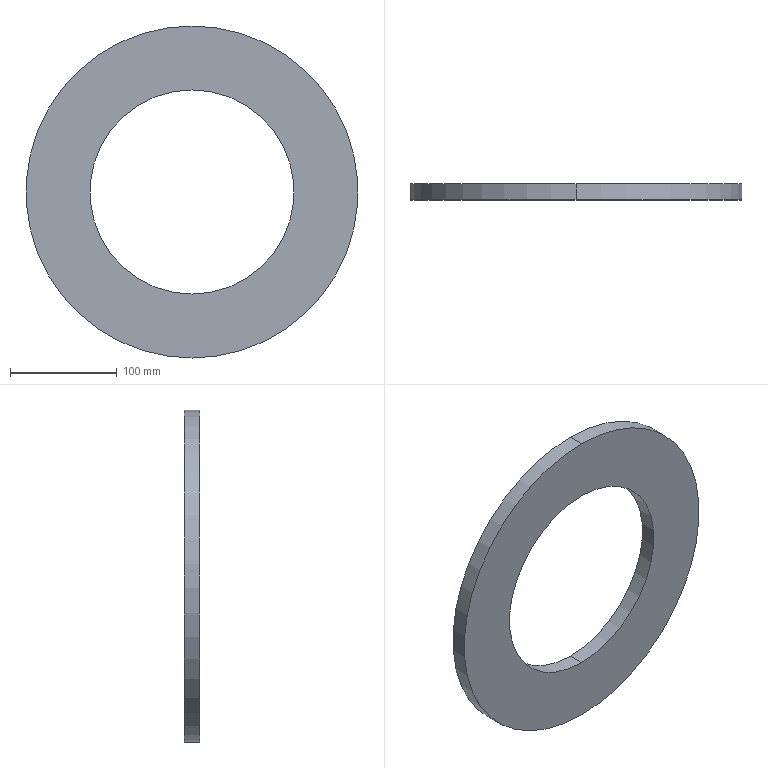Part | SolidWorks | features Extrusion 1 | 1 solid | 6 faces | box 311.64 x 15 x 311.64 mm | volume 711495 mm3 | cylinder 4 | plane 2 | commonest cylinder face diameters 191.64 x2 311.64 x2
STEP:
#1=CARTESIAN_POINT('',(0.,15.,-95.82));
#2=VERTEX_POINT('',#1);
#3=CARTESIAN_POINT('',(0.,15.,95.82));
#4=VERTEX_POINT('',#3);
#5=CARTESIAN_POINT('',(0.,15.,0.));
#6=DIRECTION('',(0.,1.,0.));
#7=DIRECTION('',(0.,0.,1.));
#8=AXIS2_PLACEMENT_3D('',#5,#6,#7);
#9=CIRCLE('',#8,95.82);
#10=EDGE_CURVE('',#2,#4,#9,.T.);
#11=ORIENTED_EDGE('',*,*,#10,.T.);
#12=CARTESIAN_POINT('',(0.,0.,95.82));
#13=VERTEX_POINT('',#12);
#14=CARTESIAN_POINT('',(0.,15.,95.82));
#15=DIRECTION('',(0.,-1.,0.));
#16=VECTOR('',#15,1000.);
#17=LINE('',#14,#16);
#18=EDGE_CURVE('',#4,#13,#17,.T.);
#19=ORIENTED_EDGE('',*,*,#18,.T.);
#20=CARTESIAN_POINT('',(0.,0.,-95.82));
#21=VERTEX_POINT('',#20);
#22=CARTESIAN_POINT('',(0.,0.,0.));
#23=DIRECTION('',(0.,1.,0.));
#24=DIRECTION('',(0.,0.,1.));
#25=AXIS2_PLACEMENT_3D('',#22,#23,#24);
#26=CIRCLE('',#25,95.82);
#27=EDGE_CURVE('',#21,#13,#26,.T.);
#28=ORIENTED_EDGE('',*,*,#27,.F.);
#29=CARTESIAN_POINT('',(0.,15.,-95.82));
#30=DIRECTION('',(0.,-1.,0.));
#31=VECTOR('',#30,1000.);
#32=LINE('',#29,#31);
#33=EDGE_CURVE('',#2,#21,#32,.T.);
#34=ORIENTED_EDGE('',*,*,#33,.F.);
#35=EDGE_LOOP('',(#11,#19,#28,#34));
#36=FACE_OUTER_BOUND('',#35,.T.);
#37=CARTESIAN_POINT('',(0.,15.,0.));
#38=DIRECTION('',(0.,-1.,0.));
#39=DIRECTION('',(0.,0.,-1.));
#40=AXIS2_PLACEMENT_3D('',#37,#38,#39);
#41=CYLINDRICAL_SURFACE('',#40,95.82);
#42=ADVANCED_FACE('',(#36),#41,.F.);
#43=CARTESIAN_POINT('',(0.,15.,155.82));
#44=VERTEX_POINT('',#43);
#45=CARTESIAN_POINT('',(0.,15.,-155.82));
#46=VERTEX_POINT('',#45);
#47=CARTESIAN_POINT('',(0.,15.,0.));
#48=DIRECTION('',(0.,1.,0.));
#49=DIRECTION('',(0.,0.,1.));
#50=AXIS2_PLACEMENT_3D('',#47,#48,#49);
#51=CIRCLE('',#50,155.82);
#52=EDGE_CURVE('',#44,#46,#51,.T.);
#53=ORIENTED_EDGE('',*,*,#52,.F.);
#54=CARTESIAN_POINT('',(0.,0.,155.82));
#55=VERTEX_POINT('',#54);
#56=CARTESIAN_POINT('',(0.,15.,155.82));
#57=DIRECTION('',(0.,-1.,0.));
#58=VECTOR('',#57,1000.);
#59=LINE('',#56,#58);
#60=EDGE_CURVE('',#44,#55,#59,.T.);
#61=ORIENTED_EDGE('',*,*,#60,.T.);
#62=CARTESIAN_POINT('',(0.,0.,-155.82));
#63=VERTEX_POINT('',#62);
#64=CARTESIAN_POINT('',(0.,0.,0.));
#65=DIRECTION('',(0.,1.,0.));
#66=DIRECTION('',(0.,0.,1.));
#67=AXIS2_PLACEMENT_3D('',#64,#65,#66);
#68=CIRCLE('',#67,155.82);
#69=EDGE_CURVE('',#55,#63,#68,.T.);
#70=ORIENTED_EDGE('',*,*,#69,.T.);
#71=CARTESIAN_POINT('',(0.,15.,-155.82));
#72=DIRECTION('',(0.,-1.,0.));
#73=VECTOR('',#72,1000.);
#74=LINE('',#71,#73);
#75=EDGE_CURVE('',#46,#63,#74,.T.);
#76=ORIENTED_EDGE('',*,*,#75,.F.);
#77=EDGE_LOOP('',(#53,#61,#70,#76));
#78=FACE_OUTER_BOUND('',#77,.T.);
#79=CARTESIAN_POINT('',(0.,15.,0.));
#80=DIRECTION('',(0.,-1.,0.));
#81=DIRECTION('',(0.,0.,-1.));
#82=AXIS2_PLACEMENT_3D('',#79,#80,#81);
#83=CYLINDRICAL_SURFACE('',#82,155.82);
#84=ADVANCED_FACE('',(#78),#83,.T.);
#85=CARTESIAN_POINT('',(0.,15.,0.));
#86=DIRECTION('',(0.,1.,0.));
#87=DIRECTION('',(0.,0.,1.));
#88=AXIS2_PLACEMENT_3D('',#85,#86,#87);
#89=CIRCLE('',#88,155.82);
#90=EDGE_CURVE('',#46,#44,#89,.T.);
#91=ORIENTED_EDGE('',*,*,#90,.T.);
#92=ORIENTED_EDGE('',*,*,#52,.T.);
#93=EDGE_LOOP('',(#91,#92));
#94=FACE_OUTER_BOUND('',#93,.T.);
#95=ORIENTED_EDGE('',*,*,#10,.F.);
#96=CARTESIAN_POINT('',(0.,15.,0.));
#97=DIRECTION('',(0.,1.,0.));
#98=DIRECTION('',(0.,0.,1.));
#99=AXIS2_PLACEMENT_3D('',#96,#97,#98);
#100=CIRCLE('',#99,95.82);
#101=EDGE_CURVE('',#4,#2,#100,.T.);
#102=ORIENTED_EDGE('',*,*,#101,.F.);
#103=EDGE_LOOP('',(#95,#102));
#104=FACE_BOUND('',#103,.T.);
#105=CARTESIAN_POINT('',(0.,15.,0.));
#106=DIRECTION('',(0.,1.,0.));
#107=DIRECTION('',(0.,0.,1.));
#108=AXIS2_PLACEMENT_3D('',#105,#106,#107);
#109=PLANE('',#108);
#110=ADVANCED_FACE('',(#94,#104),#109,.T.);
#111=CARTESIAN_POINT('',(0.,0.,0.));
#112=DIRECTION('',(0.,1.,0.));
#113=DIRECTION('',(0.,0.,1.));
#114=AXIS2_PLACEMENT_3D('',#111,#112,#113);
#115=CIRCLE('',#114,155.82);
#116=EDGE_CURVE('',#63,#55,#115,.T.);
#117=ORIENTED_EDGE('',*,*,#116,.F.);
#118=ORIENTED_EDGE('',*,*,#69,.F.);
#119=EDGE_LOOP('',(#117,#118));
#120=FACE_OUTER_BOUND('',#119,.T.);
#121=ORIENTED_EDGE('',*,*,#27,.T.);
#122=CARTESIAN_POINT('',(0.,0.,0.));
#123=DIRECTION('',(0.,1.,0.));
#124=DIRECTION('',(0.,0.,1.));
#125=AXIS2_PLACEMENT_3D('',#122,#123,#124);
#126=CIRCLE('',#125,95.82);
#127=EDGE_CURVE('',#13,#21,#126,.T.);
#128=ORIENTED_EDGE('',*,*,#127,.T.);
#129=EDGE_LOOP('',(#121,#128));
#130=FACE_BOUND('',#129,.T.);
#131=CARTESIAN_POINT('',(0.,0.,0.));
#132=DIRECTION('',(0.,1.,0.));
#133=DIRECTION('',(0.,0.,1.));
#134=AXIS2_PLACEMENT_3D('',#131,#132,#133);
#135=PLANE('',#134);
#136=ADVANCED_FACE('',(#120,#130),#135,.F.);
#137=ORIENTED_EDGE('',*,*,#60,.F.);
#138=ORIENTED_EDGE('',*,*,#90,.F.);
#139=ORIENTED_EDGE('',*,*,#75,.T.);
#140=ORIENTED_EDGE('',*,*,#116,.T.);
#141=EDGE_LOOP('',(#137,#138,#139,#140));
#142=FACE_OUTER_BOUND('',#141,.T.);
#143=CARTESIAN_POINT('',(0.,15.,0.));
#144=DIRECTION('',(0.,-1.,0.));
#145=DIRECTION('',(0.,0.,-1.));
#146=AXIS2_PLACEMENT_3D('',#143,#144,#145);
#147=CYLINDRICAL_SURFACE('',#146,155.82);
#148=ADVANCED_FACE('',(#142),#147,.T.);
#149=ORIENTED_EDGE('',*,*,#18,.F.);
#150=ORIENTED_EDGE('',*,*,#101,.T.);
#151=ORIENTED_EDGE('',*,*,#33,.T.);
#152=ORIENTED_EDGE('',*,*,#127,.F.);
#153=EDGE_LOOP('',(#149,#150,#151,#152));
#154=FACE_OUTER_BOUND('',#153,.T.);
#155=CARTESIAN_POINT('',(0.,15.,0.));
#156=DIRECTION('',(0.,-1.,0.));
#157=DIRECTION('',(0.,0.,-1.));
#158=AXIS2_PLACEMENT_3D('',#155,#156,#157);
#159=CYLINDRICAL_SURFACE('',#158,95.82);
#160=ADVANCED_FACE('',(#154),#159,.F.);
#161=CLOSED_SHELL('',(#42,#84,#110,#136,#148,#160));
#162=MANIFOLD_SOLID_BREP('',#161);
#163=CARTESIAN_POINT('',(0.,0.,0.));
#164=DIRECTION('',(0.,0.,1.));
#165=DIRECTION('',(1.,0.,0.));
#166=AXIS2_PLACEMENT_3D('',#163,#164,#165);
#167=(LENGTH_UNIT()NAMED_UNIT(*)SI_UNIT(.MILLI.,.METRE.));
#168=UNCERTAINTY_MEASURE_WITH_UNIT(LENGTH_MEASURE(0.00001),#167,'','');
#169=(NAMED_UNIT(*)PLANE_ANGLE_UNIT()SI_UNIT($,.RADIAN.));
#170=(NAMED_UNIT(*)SI_UNIT($,.STERADIAN.)SOLID_ANGLE_UNIT());
#171=(GEOMETRIC_REPRESENTATION_CONTEXT(3)GLOBAL_UNCERTAINTY_ASSIGNED_CONTEXT((#168))GLOBAL_UNIT_ASSIGNED_CONTEXT((#167,#169,#170))REPRESENTATION_CONTEXT('',''));
#172=ADVANCED_BREP_SHAPE_REPRESENTATION('',(#162,#166),#171);